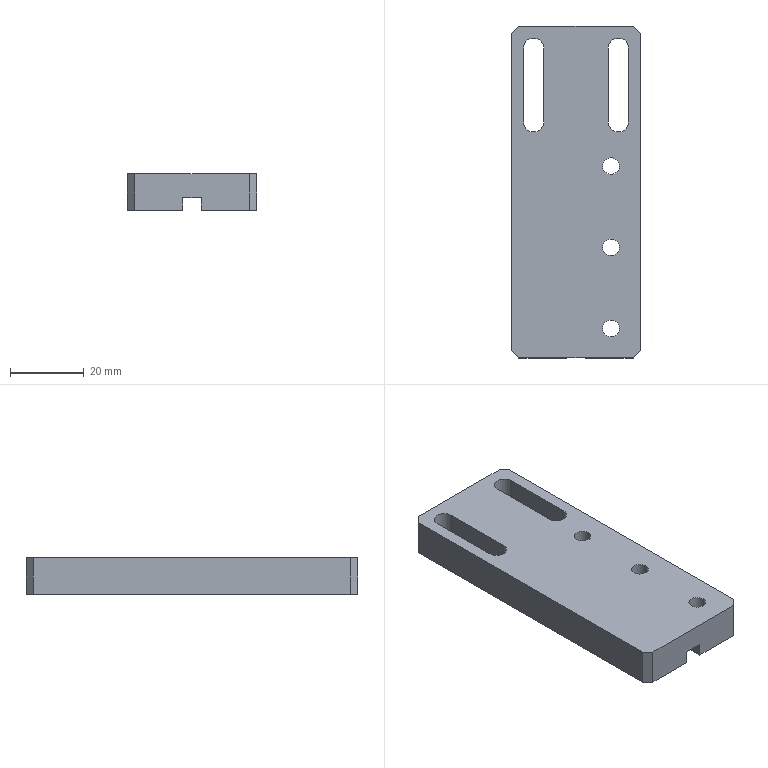Part | STEP file | 11-FG-B03611 | 1 solid | 37 faces | box 35 x 90 x 10 mm | volume 26239 mm3 | plane 21 | cylinder 16 | commonest cylinder face diameters 4.5 x6 8 x6 5.5 x4
STEP:
#1=CARTESIAN_POINT('',(13.5,-37.,4.4));
#2=VERTEX_POINT('',#1);
#3=CARTESIAN_POINT('',(5.5,-37.,4.4));
#4=VERTEX_POINT('',#3);
#5=CARTESIAN_POINT('',(9.5,-37.,4.4));
#6=DIRECTION('',(0.,0.,-1.));
#7=DIRECTION('',(-1.,0.,0.));
#8=AXIS2_PLACEMENT_3D('',#5,#6,#7);
#9=CIRCLE('',#8,4.);
#10=EDGE_CURVE('',#2,#4,#9,.T.);
#11=ORIENTED_EDGE('',*,*,#10,.F.);
#12=CARTESIAN_POINT('',(13.5,-37.,0.));
#13=VERTEX_POINT('',#12);
#14=CARTESIAN_POINT('',(13.5,-37.,0.));
#15=DIRECTION('',(0.,0.,-1.));
#16=VECTOR('',#15,1000.);
#17=LINE('',#14,#16);
#18=EDGE_CURVE('',#2,#13,#17,.T.);
#19=ORIENTED_EDGE('',*,*,#18,.T.);
#20=CARTESIAN_POINT('',(5.5,-37.,0.));
#21=VERTEX_POINT('',#20);
#22=CARTESIAN_POINT('',(9.5,-37.,0.));
#23=DIRECTION('',(0.,0.,-1.));
#24=DIRECTION('',(-1.,0.,0.));
#25=AXIS2_PLACEMENT_3D('',#22,#23,#24);
#26=CIRCLE('',#25,4.);
#27=EDGE_CURVE('',#13,#21,#26,.T.);
#28=ORIENTED_EDGE('',*,*,#27,.T.);
#29=CARTESIAN_POINT('',(5.5,-37.,0.));
#30=DIRECTION('',(0.,0.,-1.));
#31=VECTOR('',#30,1000.);
#32=LINE('',#29,#31);
#33=EDGE_CURVE('',#4,#21,#32,.T.);
#34=ORIENTED_EDGE('',*,*,#33,.F.);
#35=EDGE_LOOP('',(#11,#19,#28,#34));
#36=FACE_OUTER_BOUND('',#35,.T.);
#37=CARTESIAN_POINT('',(9.5,-37.,0.));
#38=DIRECTION('',(0.,0.,-1.));
#39=DIRECTION('',(-1.,0.,0.));
#40=AXIS2_PLACEMENT_3D('',#37,#38,#39);
#41=CYLINDRICAL_SURFACE('',#40,4.);
#42=ADVANCED_FACE('',(#36),#41,.F.);
#43=CARTESIAN_POINT('',(11.75,-37.,10.));
#44=VERTEX_POINT('',#43);
#45=CARTESIAN_POINT('',(7.25,-37.,10.));
#46=VERTEX_POINT('',#45);
#47=CARTESIAN_POINT('',(9.5,-37.,10.));
#48=DIRECTION('',(0.,0.,-1.));
#49=DIRECTION('',(-1.,0.,0.));
#50=AXIS2_PLACEMENT_3D('',#47,#48,#49);
#51=CIRCLE('',#50,2.25);
#52=EDGE_CURVE('',#44,#46,#51,.T.);
#53=ORIENTED_EDGE('',*,*,#52,.F.);
#54=CARTESIAN_POINT('',(11.75,-37.,4.4));
#55=VERTEX_POINT('',#54);
#56=CARTESIAN_POINT('',(11.75,-37.,0.));
#57=DIRECTION('',(0.,0.,-1.));
#58=VECTOR('',#57,1000.);
#59=LINE('',#56,#58);
#60=EDGE_CURVE('',#44,#55,#59,.T.);
#61=ORIENTED_EDGE('',*,*,#60,.T.);
#62=CARTESIAN_POINT('',(7.25,-37.,4.4));
#63=VERTEX_POINT('',#62);
#64=CARTESIAN_POINT('',(9.5,-37.,4.4));
#65=DIRECTION('',(0.,0.,-1.));
#66=DIRECTION('',(-1.,0.,0.));
#67=AXIS2_PLACEMENT_3D('',#64,#65,#66);
#68=CIRCLE('',#67,2.25);
#69=EDGE_CURVE('',#55,#63,#68,.T.);
#70=ORIENTED_EDGE('',*,*,#69,.T.);
#71=CARTESIAN_POINT('',(7.25,-37.,0.));
#72=DIRECTION('',(0.,0.,-1.));
#73=VECTOR('',#72,1000.);
#74=LINE('',#71,#73);
#75=EDGE_CURVE('',#46,#63,#74,.T.);
#76=ORIENTED_EDGE('',*,*,#75,.F.);
#77=EDGE_LOOP('',(#53,#61,#70,#76));
#78=FACE_OUTER_BOUND('',#77,.T.);
#79=CARTESIAN_POINT('',(9.5,-37.,0.));
#80=DIRECTION('',(0.,0.,-1.));
#81=DIRECTION('',(-1.,0.,0.));
#82=AXIS2_PLACEMENT_3D('',#79,#80,#81);
#83=CYLINDRICAL_SURFACE('',#82,2.25);
#84=ADVANCED_FACE('',(#78),#83,.F.);
#85=CARTESIAN_POINT('',(13.5,-15.,4.4));
#86=VERTEX_POINT('',#85);
#87=CARTESIAN_POINT('',(5.5,-15.,4.4));
#88=VERTEX_POINT('',#87);
#89=CARTESIAN_POINT('',(9.5,-15.,4.4));
#90=DIRECTION('',(0.,0.,-1.));
#91=DIRECTION('',(-1.,0.,0.));
#92=AXIS2_PLACEMENT_3D('',#89,#90,#91);
#93=CIRCLE('',#92,4.);
#94=EDGE_CURVE('',#86,#88,#93,.T.);
#95=ORIENTED_EDGE('',*,*,#94,.F.);
#96=CARTESIAN_POINT('',(13.5,-15.,0.));
#97=VERTEX_POINT('',#96);
#98=CARTESIAN_POINT('',(13.5,-15.,0.));
#99=DIRECTION('',(0.,0.,-1.));
#100=VECTOR('',#99,1000.);
#101=LINE('',#98,#100);
#102=EDGE_CURVE('',#86,#97,#101,.T.);
#103=ORIENTED_EDGE('',*,*,#102,.T.);
#104=CARTESIAN_POINT('',(5.5,-15.,0.));
#105=VERTEX_POINT('',#104);
#106=CARTESIAN_POINT('',(9.5,-15.,0.));
#107=DIRECTION('',(0.,0.,-1.));
#108=DIRECTION('',(-1.,0.,0.));
#109=AXIS2_PLACEMENT_3D('',#106,#107,#108);
#110=CIRCLE('',#109,4.);
#111=EDGE_CURVE('',#97,#105,#110,.T.);
#112=ORIENTED_EDGE('',*,*,#111,.T.);
#113=CARTESIAN_POINT('',(5.5,-15.,0.));
#114=DIRECTION('',(0.,0.,-1.));
#115=VECTOR('',#114,1000.);
#116=LINE('',#113,#115);
#117=EDGE_CURVE('',#88,#105,#116,.T.);
#118=ORIENTED_EDGE('',*,*,#117,.F.);
#119=EDGE_LOOP('',(#95,#103,#112,#118));
#120=FACE_OUTER_BOUND('',#119,.T.);
#121=CARTESIAN_POINT('',(9.5,-15.,0.));
#122=DIRECTION('',(0.,0.,-1.));
#123=DIRECTION('',(-1.,0.,0.));
#124=AXIS2_PLACEMENT_3D('',#121,#122,#123);
#125=CYLINDRICAL_SURFACE('',#124,4.);
#126=ADVANCED_FACE('',(#120),#125,.F.);
#127=CARTESIAN_POINT('',(11.75,-15.,10.));
#128=VERTEX_POINT('',#127);
#129=CARTESIAN_POINT('',(7.25,-15.,10.));
#130=VERTEX_POINT('',#129);
#131=CARTESIAN_POINT('',(9.5,-15.,10.));
#132=DIRECTION('',(0.,0.,-1.));
#133=DIRECTION('',(-1.,0.,0.));
#134=AXIS2_PLACEMENT_3D('',#131,#132,#133);
#135=CIRCLE('',#134,2.25);
#136=EDGE_CURVE('',#128,#130,#135,.T.);
#137=ORIENTED_EDGE('',*,*,#136,.F.);
#138=CARTESIAN_POINT('',(11.75,-15.,4.4));
#139=VERTEX_POINT('',#138);
#140=CARTESIAN_POINT('',(11.75,-15.,0.));
#141=DIRECTION('',(0.,0.,-1.));
#142=VECTOR('',#141,1000.);
#143=LINE('',#140,#142);
#144=EDGE_CURVE('',#128,#139,#143,.T.);
#145=ORIENTED_EDGE('',*,*,#144,.T.);
#146=CARTESIAN_POINT('',(7.25,-15.,4.4));
#147=VERTEX_POINT('',#146);
#148=CARTESIAN_POINT('',(9.5,-15.,4.4));
#149=DIRECTION('',(0.,0.,-1.));
#150=DIRECTION('',(-1.,0.,0.));
#151=AXIS2_PLACEMENT_3D('',#148,#149,#150);
#152=CIRCLE('',#151,2.25);
#153=EDGE_CURVE('',#139,#147,#152,.T.);
#154=ORIENTED_EDGE('',*,*,#153,.T.);
#155=CARTESIAN_POINT('',(7.25,-15.,0.));
#156=DIRECTION('',(0.,0.,-1.));
#157=VECTOR('',#156,1000.);
#158=LINE('',#155,#157);
#159=EDGE_CURVE('',#130,#147,#158,.T.);
#160=ORIENTED_EDGE('',*,*,#159,.F.);
#161=EDGE_LOOP('',(#137,#145,#154,#160));
#162=FACE_OUTER_BOUND('',#161,.T.);
#163=CARTESIAN_POINT('',(9.5,-15.,0.));
#164=DIRECTION('',(0.,0.,-1.));
#165=DIRECTION('',(-1.,0.,0.));
#166=AXIS2_PLACEMENT_3D('',#163,#164,#165);
#167=CYLINDRICAL_SURFACE('',#166,2.25);
#168=ADVANCED_FACE('',(#162),#167,.F.);
#169=CARTESIAN_POINT('',(13.5,7.,4.4));
#170=VERTEX_POINT('',#169);
#171=CARTESIAN_POINT('',(5.5,7.,4.4));
#172=VERTEX_POINT('',#171);
#173=CARTESIAN_POINT('',(9.5,7.,4.4));
#174=DIRECTION('',(0.,0.,-1.));
#175=DIRECTION('',(-1.,0.,0.));
#176=AXIS2_PLACEMENT_3D('',#173,#174,#175);
#177=CIRCLE('',#176,4.);
#178=EDGE_CURVE('',#170,#172,#177,.T.);
#179=ORIENTED_EDGE('',*,*,#178,.F.);
#180=CARTESIAN_POINT('',(13.5,7.,0.));
#181=VERTEX_POINT('',#180);
#182=CARTESIAN_POINT('',(13.5,7.,0.));
#183=DIRECTION('',(0.,0.,-1.));
#184=VECTOR('',#183,1000.);
#185=LINE('',#182,#184);
#186=EDGE_CURVE('',#170,#181,#185,.T.);
#187=ORIENTED_EDGE('',*,*,#186,.T.);
#188=CARTESIAN_POINT('',(5.5,7.,0.));
#189=VERTEX_POINT('',#188);
#190=CARTESIAN_POINT('',(9.5,7.,0.));
#191=DIRECTION('',(0.,0.,-1.));
#192=DIRECTION('',(-1.,0.,0.));
#193=AXIS2_PLACEMENT_3D('',#190,#191,#192);
#194=CIRCLE('',#193,4.);
#195=EDGE_CURVE('',#181,#189,#194,.T.);
#196=ORIENTED_EDGE('',*,*,#195,.T.);
#197=CARTESIAN_POINT('',(5.5,7.,0.));
#198=DIRECTION('',(0.,0.,-1.));
#199=VECTOR('',#198,1000.);
#200=LINE('',#197,#199);
#201=EDGE_CURVE('',#172,#189,#200,.T.);
#202=ORIENTED_EDGE('',*,*,#201,.F.);
#203=EDGE_LOOP('',(#179,#187,#196,#202));
#204=FACE_OUTER_BOUND('',#203,.T.);
#205=CARTESIAN_POINT('',(9.5,7.,0.));
#206=DIRECTION('',(0.,0.,-1.));
#207=DIRECTION('',(-1.,0.,0.));
#208=AXIS2_PLACEMENT_3D('',#205,#206,#207);
#209=CYLINDRICAL_SURFACE('',#208,4.);
#210=ADVANCED_FACE('',(#204),#209,.F.);
#211=CARTESIAN_POINT('',(11.75,7.,10.));
#212=VERTEX_POINT('',#211);
#213=CARTESIAN_POINT('',(7.25,7.,10.));
#214=VERTEX_POINT('',#213);
#215=CARTESIAN_POINT('',(9.5,7.,10.));
#216=DIRECTION('',(0.,0.,-1.));
#217=DIRECTION('',(-1.,0.,0.));
#218=AXIS2_PLACEMENT_3D('',#215,#216,#217);
#219=CIRCLE('',#218,2.25);
#220=EDGE_CURVE('',#212,#214,#219,.T.);
#221=ORIENTED_EDGE('',*,*,#220,.F.);
#222=CARTESIAN_POINT('',(11.75,7.,4.4));
#223=VERTEX_POINT('',#222);
#224=CARTESIAN_POINT('',(11.75,7.,0.));
#225=DIRECTION('',(0.,0.,-1.));
#226=VECTOR('',#225,1000.);
#227=LINE('',#224,#226);
#228=EDGE_CURVE('',#212,#223,#227,.T.);
#229=ORIENTED_EDGE('',*,*,#228,.T.);
#230=CARTESIAN_POINT('',(7.25,7.,4.4));
#231=VERTEX_POINT('',#230);
#232=CARTESIAN_POINT('',(9.5,7.,4.4));
#233=DIRECTION('',(0.,0.,-1.));
#234=DIRECTION('',(-1.,0.,0.));
#235=AXIS2_PLACEMENT_3D('',#232,#233,#234);
#236=CIRCLE('',#235,2.25);
#237=EDGE_CURVE('',#223,#231,#236,.T.);
#238=ORIENTED_EDGE('',*,*,#237,.T.);
#239=CARTESIAN_POINT('',(7.25,7.,0.));
#240=DIRECTION('',(0.,0.,-1.));
#241=VECTOR('',#240,1000.);
#242=LINE('',#239,#241);
#243=EDGE_CURVE('',#214,#231,#242,.T.);
#244=ORIENTED_EDGE('',*,*,#243,.F.);
#245=EDGE_LOOP('',(#221,#229,#238,#244));
#246=FACE_OUTER_BOUND('',#245,.T.);
#247=CARTESIAN_POINT('',(9.5,7.,0.));
#248=DIRECTION('',(0.,0.,-1.));
#249=DIRECTION('',(-1.,0.,0.));
#250=AXIS2_PLACEMENT_3D('',#247,#248,#249);
#251=CYLINDRICAL_SURFACE('',#250,2.25);
#252=ADVANCED_FACE('',(#246),#251,.F.);
#253=CARTESIAN_POINT('',(14.25,19.,0.));
#254=VERTEX_POINT('',#253);
#255=CARTESIAN_POINT('',(8.75,19.,0.));
#256=VERTEX_POINT('',#255);
#257=CARTESIAN_POINT('',(11.5,19.,0.));
#258=DIRECTION('',(0.,0.,-1.));
#259=DIRECTION('',(-1.,0.,0.));
#260=AXIS2_PLACEMENT_3D('',#257,#258,#259);
#261=CIRCLE('',#260,2.75);
#262=EDGE_CURVE('',#254,#256,#261,.T.);
#263=ORIENTED_EDGE('',*,*,#262,.F.);
#264=CARTESIAN_POINT('',(14.25,39.,0.));
#265=VERTEX_POINT('',#264);
#266=CARTESIAN_POINT('',(14.25,0.,0.));
#267=DIRECTION('',(0.,-1.,0.));
#268=VECTOR('',#267,1000.);
#269=LINE('',#266,#268);
#270=EDGE_CURVE('',#265,#254,#269,.T.);
#271=ORIENTED_EDGE('',*,*,#270,.F.);
#272=CARTESIAN_POINT('',(8.75,39.,0.));
#273=VERTEX_POINT('',#272);
#274=CARTESIAN_POINT('',(11.5,39.,0.));
#275=DIRECTION('',(0.,0.,-1.));
#276=DIRECTION('',(-1.,0.,0.));
#277=AXIS2_PLACEMENT_3D('',#274,#275,#276);
#278=CIRCLE('',#277,2.75);
#279=EDGE_CURVE('',#273,#265,#278,.T.);
#280=ORIENTED_EDGE('',*,*,#279,.F.);
#281=CARTESIAN_POINT('',(8.75,0.,0.));
#282=DIRECTION('',(0.,1.,0.));
#283=VECTOR('',#282,1000.);
#284=LINE('',#281,#283);
#285=EDGE_CURVE('',#256,#273,#284,.T.);
#286=ORIENTED_EDGE('',*,*,#285,.F.);
#287=EDGE_LOOP('',(#263,#271,#280,#286));
#288=FACE_BOUND('',#287,.T.);
#289=CARTESIAN_POINT('',(2.5,45.,0.));
#290=VERTEX_POINT('',#289);
#291=CARTESIAN_POINT('',(2.5,-45.,0.));
#292=VERTEX_POINT('',#291);
#293=CARTESIAN_POINT('',(2.5,0.,0.));
#294=DIRECTION('',(0.,-1.,0.));
#295=VECTOR('',#294,1000.);
#296=LINE('',#293,#295);
#297=EDGE_CURVE('',#290,#292,#296,.T.);
#298=ORIENTED_EDGE('',*,*,#297,.F.);
#299=CARTESIAN_POINT('',(15.5,45.,0.));
#300=VERTEX_POINT('',#299);
#301=CARTESIAN_POINT('',(17.5,45.,0.));
#302=DIRECTION('',(-1.,0.,0.));
#303=VECTOR('',#302,1000.);
#304=LINE('',#301,#303);
#305=EDGE_CURVE('',#300,#290,#304,.T.);
#306=ORIENTED_EDGE('',*,*,#305,.F.);
#307=CARTESIAN_POINT('',(17.5,43.,0.));
#308=VERTEX_POINT('',#307);
#309=CARTESIAN_POINT('',(30.25,30.25,0.));
#310=DIRECTION('',(0.7071,-0.7071,0.));
#311=VECTOR('',#310,1000.);
#312=LINE('',#309,#311);
#313=EDGE_CURVE('',#300,#308,#312,.T.);
#314=ORIENTED_EDGE('',*,*,#313,.T.);
#315=CARTESIAN_POINT('',(17.5,-43.,0.));
#316=VERTEX_POINT('',#315);
#317=CARTESIAN_POINT('',(17.5,45.,0.));
#318=DIRECTION('',(0.,1.,0.));
#319=VECTOR('',#318,1000.);
#320=LINE('',#317,#319);
#321=EDGE_CURVE('',#316,#308,#320,.T.);
#322=ORIENTED_EDGE('',*,*,#321,.F.);
#323=CARTESIAN_POINT('',(15.5,-45.,0.));
#324=VERTEX_POINT('',#323);
#325=CARTESIAN_POINT('',(30.25,-30.25,0.));
#326=DIRECTION('',(-0.7071,-0.7071,0.));
#327=VECTOR('',#326,1000.);
#328=LINE('',#325,#327);
#329=EDGE_CURVE('',#316,#324,#328,.T.);
#330=ORIENTED_EDGE('',*,*,#329,.T.);
#331=CARTESIAN_POINT('',(17.5,-45.,0.));
#332=DIRECTION('',(1.,0.,0.));
#333=VECTOR('',#332,1000.);
#334=LINE('',#331,#333);
#335=EDGE_CURVE('',#292,#324,#334,.T.);
#336=ORIENTED_EDGE('',*,*,#335,.F.);
#337=EDGE_LOOP('',(#298,#306,#314,#322,#330,#336));
#338=FACE_OUTER_BOUND('',#337,.T.);
#339=CARTESIAN_POINT('',(9.5,-37.,0.));
#340=DIRECTION('',(0.,0.,-1.));
#341=DIRECTION('',(-1.,0.,0.));
#342=AXIS2_PLACEMENT_3D('',#339,#340,#341);
#343=CIRCLE('',#342,4.);
#344=EDGE_CURVE('',#21,#13,#343,.T.);
#345=ORIENTED_EDGE('',*,*,#344,.F.);
#346=ORIENTED_EDGE('',*,*,#27,.F.);
#347=EDGE_LOOP('',(#345,#346));
#348=FACE_BOUND('',#347,.T.);
#349=CARTESIAN_POINT('',(9.5,-15.,0.));
#350=DIRECTION('',(0.,0.,-1.));
#351=DIRECTION('',(-1.,0.,0.));
#352=AXIS2_PLACEMENT_3D('',#349,#350,#351);
#353=CIRCLE('',#352,4.);
#354=EDGE_CURVE('',#105,#97,#353,.T.);
#355=ORIENTED_EDGE('',*,*,#354,.F.);
#356=ORIENTED_EDGE('',*,*,#111,.F.);
#357=EDGE_LOOP('',(#355,#356));
#358=FACE_BOUND('',#357,.T.);
#359=CARTESIAN_POINT('',(9.5,7.,0.));
#360=DIRECTION('',(0.,0.,-1.));
#361=DIRECTION('',(-1.,0.,0.));
#362=AXIS2_PLACEMENT_3D('',#359,#360,#361);
#363=CIRCLE('',#362,4.);
#364=EDGE_CURVE('',#189,#181,#363,.T.);
#365=ORIENTED_EDGE('',*,*,#364,.F.);
#366=ORIENTED_EDGE('',*,*,#195,.F.);
#367=EDGE_LOOP('',(#365,#366));
#368=FACE_BOUND('',#367,.T.);
#369=CARTESIAN_POINT('',(0.,0.,0.));
#370=DIRECTION('',(0.,0.,-1.));
#371=DIRECTION('',(-1.,0.,0.));
#372=AXIS2_PLACEMENT_3D('',#369,#370,#371);
#373=PLANE('',#372);
#374=ADVANCED_FACE('',(#288,#338,#348,#358,#368),#373,.T.);
#375=CARTESIAN_POINT('',(-17.5,43.,10.));
#376=VERTEX_POINT('',#375);
#377=CARTESIAN_POINT('',(-17.5,-43.,10.));
#378=VERTEX_POINT('',#377);
#379=CARTESIAN_POINT('',(-17.5,45.,10.));
#380=DIRECTION('',(0.,-1.,0.));
#381=VECTOR('',#380,1000.);
#382=LINE('',#379,#381);
#383=EDGE_CURVE('',#376,#378,#382,.T.);
#384=ORIENTED_EDGE('',*,*,#383,.F.);
#385=CARTESIAN_POINT('',(-17.5,43.,0.));
#386=VERTEX_POINT('',#385);
#387=CARTESIAN_POINT('',(-17.5,43.,10.));
#388=DIRECTION('',(0.,0.,-1.));
#389=VECTOR('',#388,1000.);
#390=LINE('',#387,#389);
#391=EDGE_CURVE('',#376,#386,#390,.T.);
#392=ORIENTED_EDGE('',*,*,#391,.T.);
#393=CARTESIAN_POINT('',(-17.5,-43.,0.));
#394=VERTEX_POINT('',#393);
#395=CARTESIAN_POINT('',(-17.5,45.,0.));
#396=DIRECTION('',(0.,-1.,0.));
#397=VECTOR('',#396,1000.);
#398=LINE('',#395,#397);
#399=EDGE_CURVE('',#386,#394,#398,.T.);
#400=ORIENTED_EDGE('',*,*,#399,.T.);
#401=CARTESIAN_POINT('',(-17.5,-43.,10.));
#402=DIRECTION('',(0.,0.,1.));
#403=VECTOR('',#402,1000.);
#404=LINE('',#401,#403);
#405=EDGE_CURVE('',#394,#378,#404,.T.);
#406=ORIENTED_EDGE('',*,*,#405,.T.);
#407=EDGE_LOOP('',(#384,#392,#400,#406));
#408=FACE_OUTER_BOUND('',#407,.T.);
#409=CARTESIAN_POINT('',(-17.5,45.,10.));
#410=DIRECTION('',(1.,0.,0.));
#411=DIRECTION('',(0.,1.,0.));
#412=AXIS2_PLACEMENT_3D('',#409,#410,#411);
#413=PLANE('',#412);
#414=ADVANCED_FACE('',(#408),#413,.F.);
#415=CARTESIAN_POINT('',(2.5,-45.,3.5));
#416=VERTEX_POINT('',#415);
#417=CARTESIAN_POINT('',(-2.5,-45.,3.5));
#418=VERTEX_POINT('',#417);
#419=CARTESIAN_POINT('',(-2.5,-45.,3.5));
#420=DIRECTION('',(-1.,0.,0.));
#421=VECTOR('',#420,1000.);
#422=LINE('',#419,#421);
#423=EDGE_CURVE('',#416,#418,#422,.T.);
#424=ORIENTED_EDGE('',*,*,#423,.F.);
#425=CARTESIAN_POINT('',(2.5,-45.,3.5));
#426=DIRECTION('',(0.,0.,1.));
#427=VECTOR('',#426,1000.);
#428=LINE('',#425,#427);
#429=EDGE_CURVE('',#292,#416,#428,.T.);
#430=ORIENTED_EDGE('',*,*,#429,.F.);
#431=ORIENTED_EDGE('',*,*,#335,.T.);
#432=CARTESIAN_POINT('',(15.5,-45.,10.));
#433=VERTEX_POINT('',#432);
#434=CARTESIAN_POINT('',(15.5,-45.,10.));
#435=DIRECTION('',(0.,0.,1.));
#436=VECTOR('',#435,1000.);
#437=LINE('',#434,#436);
#438=EDGE_CURVE('',#324,#433,#437,.T.);
#439=ORIENTED_EDGE('',*,*,#438,.T.);
#440=CARTESIAN_POINT('',(-15.5,-45.,10.));
#441=VERTEX_POINT('',#440);
#442=CARTESIAN_POINT('',(17.5,-45.,10.));
#443=DIRECTION('',(1.,0.,0.));
#444=VECTOR('',#443,1000.);
#445=LINE('',#442,#444);
#446=EDGE_CURVE('',#441,#433,#445,.T.);
#447=ORIENTED_EDGE('',*,*,#446,.F.);
#448=CARTESIAN_POINT('',(-15.5,-45.,0.));
#449=VERTEX_POINT('',#448);
#450=CARTESIAN_POINT('',(-15.5,-45.,10.));
#451=DIRECTION('',(0.,0.,-1.));
#452=VECTOR('',#451,1000.);
#453=LINE('',#450,#452);
#454=EDGE_CURVE('',#441,#449,#453,.T.);
#455=ORIENTED_EDGE('',*,*,#454,.T.);
#456=CARTESIAN_POINT('',(-2.5,-45.,0.));
#457=VERTEX_POINT('',#456);
#458=CARTESIAN_POINT('',(17.5,-45.,0.));
#459=DIRECTION('',(1.,0.,0.));
#460=VECTOR('',#459,1000.);
#461=LINE('',#458,#460);
#462=EDGE_CURVE('',#449,#457,#461,.T.);
#463=ORIENTED_EDGE('',*,*,#462,.T.);
#464=CARTESIAN_POINT('',(-2.5,-45.,3.5));
#465=DIRECTION('',(0.,0.,-1.));
#466=VECTOR('',#465,1000.);
#467=LINE('',#464,#466);
#468=EDGE_CURVE('',#418,#457,#467,.T.);
#469=ORIENTED_EDGE('',*,*,#468,.F.);
#470=EDGE_LOOP('',(#424,#430,#431,#439,#447,#455,#463,#469));
#471=FACE_OUTER_BOUND('',#470,.T.);
#472=CARTESIAN_POINT('',(17.5,-45.,10.));
#473=DIRECTION('',(0.,1.,0.));
#474=DIRECTION('',(-1.,0.,0.));
#475=AXIS2_PLACEMENT_3D('',#472,#473,#474);
#476=PLANE('',#475);
#477=ADVANCED_FACE('',(#471),#476,.F.);
#478=ORIENTED_EDGE('',*,*,#321,.T.);
#479=CARTESIAN_POINT('',(17.5,43.,10.));
#480=VERTEX_POINT('',#479);
#481=CARTESIAN_POINT('',(17.5,43.,10.));
#482=DIRECTION('',(0.,0.,1.));
#483=VECTOR('',#482,1000.);
#484=LINE('',#481,#483);
#485=EDGE_CURVE('',#308,#480,#484,.T.);
#486=ORIENTED_EDGE('',*,*,#485,.T.);
#487=CARTESIAN_POINT('',(17.5,-43.,10.));
#488=VERTEX_POINT('',#487);
#489=CARTESIAN_POINT('',(17.5,45.,10.));
#490=DIRECTION('',(0.,1.,0.));
#491=VECTOR('',#490,1000.);
#492=LINE('',#489,#491);
#493=EDGE_CURVE('',#488,#480,#492,.T.);
#494=ORIENTED_EDGE('',*,*,#493,.F.);
#495=CARTESIAN_POINT('',(17.5,-43.,10.));
#496=DIRECTION('',(0.,0.,-1.));
#497=VECTOR('',#496,1000.);
#498=LINE('',#495,#497);
#499=EDGE_CURVE('',#488,#316,#498,.T.);
#500=ORIENTED_EDGE('',*,*,#499,.T.);
#501=EDGE_LOOP('',(#478,#486,#494,#500));
#502=FACE_OUTER_BOUND('',#501,.T.);
#503=CARTESIAN_POINT('',(17.5,45.,10.));
#504=DIRECTION('',(-1.,0.,0.));
#505=DIRECTION('',(0.,-1.,0.));
#506=AXIS2_PLACEMENT_3D('',#503,#504,#505);
#507=PLANE('',#506);
#508=ADVANCED_FACE('',(#502),#507,.F.);
#509=ORIENTED_EDGE('',*,*,#305,.T.);
#510=CARTESIAN_POINT('',(2.5,45.,3.5));
#511=VERTEX_POINT('',#510);
#512=CARTESIAN_POINT('',(2.5,45.,10.));
#513=DIRECTION('',(0.,0.,1.));
#514=VECTOR('',#513,1000.);
#515=LINE('',#512,#514);
#516=EDGE_CURVE('',#290,#511,#515,.T.);
#517=ORIENTED_EDGE('',*,*,#516,.T.);
#518=CARTESIAN_POINT('',(-2.5,45.,3.5));
#519=VERTEX_POINT('',#518);
#520=CARTESIAN_POINT('',(17.5,45.,3.5));
#521=DIRECTION('',(-1.,0.,0.));
#522=VECTOR('',#521,1000.);
#523=LINE('',#520,#522);
#524=EDGE_CURVE('',#511,#519,#523,.T.);
#525=ORIENTED_EDGE('',*,*,#524,.T.);
#526=CARTESIAN_POINT('',(-2.5,45.,0.));
#527=VERTEX_POINT('',#526);
#528=CARTESIAN_POINT('',(-2.5,45.,10.));
#529=DIRECTION('',(0.,0.,-1.));
#530=VECTOR('',#529,1000.);
#531=LINE('',#528,#530);
#532=EDGE_CURVE('',#519,#527,#531,.T.);
#533=ORIENTED_EDGE('',*,*,#532,.T.);
#534=CARTESIAN_POINT('',(-15.5,45.,0.));
#535=VERTEX_POINT('',#534);
#536=CARTESIAN_POINT('',(17.5,45.,0.));
#537=DIRECTION('',(-1.,0.,0.));
#538=VECTOR('',#537,1000.);
#539=LINE('',#536,#538);
#540=EDGE_CURVE('',#527,#535,#539,.T.);
#541=ORIENTED_EDGE('',*,*,#540,.T.);
#542=CARTESIAN_POINT('',(-15.5,45.,10.));
#543=VERTEX_POINT('',#542);
#544=CARTESIAN_POINT('',(-15.5,45.,10.));
#545=DIRECTION('',(0.,0.,1.));
#546=VECTOR('',#545,1000.);
#547=LINE('',#544,#546);
#548=EDGE_CURVE('',#535,#543,#547,.T.);
#549=ORIENTED_EDGE('',*,*,#548,.T.);
#550=CARTESIAN_POINT('',(15.5,45.,10.));
#551=VERTEX_POINT('',#550);
#552=CARTESIAN_POINT('',(17.5,45.,10.));
#553=DIRECTION('',(-1.,0.,0.));
#554=VECTOR('',#553,1000.);
#555=LINE('',#552,#554);
#556=EDGE_CURVE('',#551,#543,#555,.T.);
#557=ORIENTED_EDGE('',*,*,#556,.F.);
#558=CARTESIAN_POINT('',(15.5,45.,10.));
#559=DIRECTION('',(0.,0.,-1.));
#560=VECTOR('',#559,1000.);
#561=LINE('',#558,#560);
#562=EDGE_CURVE('',#551,#300,#561,.T.);
#563=ORIENTED_EDGE('',*,*,#562,.T.);
#564=EDGE_LOOP('',(#509,#517,#525,#533,#541,#549,#557,#563));
#565=FACE_OUTER_BOUND('',#564,.T.);
#566=CARTESIAN_POINT('',(17.5,45.,10.));
#567=DIRECTION('',(0.,-1.,0.));
#568=DIRECTION('',(1.,0.,0.));
#569=AXIS2_PLACEMENT_3D('',#566,#567,#568);
#570=PLANE('',#569);
#571=ADVANCED_FACE('',(#565),#570,.F.);
#572=CARTESIAN_POINT('',(-8.75,19.,10.));
#573=VERTEX_POINT('',#572);
#574=CARTESIAN_POINT('',(-8.75,39.,10.));
#575=VERTEX_POINT('',#574);
#576=CARTESIAN_POINT('',(-8.75,19.,10.));
#577=DIRECTION('',(0.,1.,0.));
#578=VECTOR('',#577,1000.);
#579=LINE('',#576,#578);
#580=EDGE_CURVE('',#573,#575,#579,.T.);
#581=ORIENTED_EDGE('',*,*,#580,.F.);
#582=CARTESIAN_POINT('',(-14.25,19.,10.));
#583=VERTEX_POINT('',#582);
#584=CARTESIAN_POINT('',(-11.5,19.,10.));
#585=DIRECTION('',(0.,0.,1.));
#586=DIRECTION('',(1.,0.,0.));
#587=AXIS2_PLACEMENT_3D('',#584,#585,#586);
#588=CIRCLE('',#587,2.75);
#589=EDGE_CURVE('',#583,#573,#588,.T.);
#590=ORIENTED_EDGE('',*,*,#589,.F.);
#591=CARTESIAN_POINT('',(-14.25,39.,10.));
#592=VERTEX_POINT('',#591);
#593=CARTESIAN_POINT('',(-14.25,19.,10.));
#594=DIRECTION('',(0.,-1.,0.));
#595=VECTOR('',#594,1000.);
#596=LINE('',#593,#595);
#597=EDGE_CURVE('',#592,#583,#596,.T.);
#598=ORIENTED_EDGE('',*,*,#597,.F.);
#599=CARTESIAN_POINT('',(-11.5,39.,10.));
#600=DIRECTION('',(0.,0.,1.));
#601=DIRECTION('',(1.,0.,0.));
#602=AXIS2_PLACEMENT_3D('',#599,#600,#601);
#603=CIRCLE('',#602,2.75);
#604=EDGE_CURVE('',#575,#592,#603,.T.);
#605=ORIENTED_EDGE('',*,*,#604,.F.);
#606=EDGE_LOOP('',(#581,#590,#598,#605));
#607=FACE_BOUND('',#606,.T.);
#608=CARTESIAN_POINT('',(14.25,19.,10.));
#609=VERTEX_POINT('',#608);
#610=CARTESIAN_POINT('',(14.25,39.,10.));
#611=VERTEX_POINT('',#610);
#612=CARTESIAN_POINT('',(14.25,19.,10.));
#613=DIRECTION('',(0.,1.,0.));
#614=VECTOR('',#613,1000.);
#615=LINE('',#612,#614);
#616=EDGE_CURVE('',#609,#611,#615,.T.);
#617=ORIENTED_EDGE('',*,*,#616,.F.);
#618=CARTESIAN_POINT('',(8.75,19.,10.));
#619=VERTEX_POINT('',#618);
#620=CARTESIAN_POINT('',(11.5,19.,10.));
#621=DIRECTION('',(0.,0.,1.));
#622=DIRECTION('',(1.,0.,0.));
#623=AXIS2_PLACEMENT_3D('',#620,#621,#622);
#624=CIRCLE('',#623,2.75);
#625=EDGE_CURVE('',#619,#609,#624,.T.);
#626=ORIENTED_EDGE('',*,*,#625,.F.);
#627=CARTESIAN_POINT('',(8.75,39.,10.));
#628=VERTEX_POINT('',#627);
#629=CARTESIAN_POINT('',(8.75,19.,10.));
#630=DIRECTION('',(0.,-1.,0.));
#631=VECTOR('',#630,1000.);
#632=LINE('',#629,#631);
#633=EDGE_CURVE('',#628,#619,#632,.T.);
#634=ORIENTED_EDGE('',*,*,#633,.F.);
#635=CARTESIAN_POINT('',(11.5,39.,10.));
#636=DIRECTION('',(0.,0.,1.));
#637=DIRECTION('',(1.,0.,0.));
#638=AXIS2_PLACEMENT_3D('',#635,#636,#637);
#639=CIRCLE('',#638,2.75);
#640=EDGE_CURVE('',#611,#628,#639,.T.);
#641=ORIENTED_EDGE('',*,*,#640,.F.);
#642=EDGE_LOOP('',(#617,#626,#634,#641));
#643=FACE_BOUND('',#642,.T.);
#644=CARTESIAN_POINT('',(9.5,-37.,10.));
#645=DIRECTION('',(0.,0.,-1.));
#646=DIRECTION('',(-1.,0.,0.));
#647=AXIS2_PLACEMENT_3D('',#644,#645,#646);
#648=CIRCLE('',#647,2.25);
#649=EDGE_CURVE('',#46,#44,#648,.T.);
#650=ORIENTED_EDGE('',*,*,#649,.T.);
#651=ORIENTED_EDGE('',*,*,#52,.T.);
#652=EDGE_LOOP('',(#650,#651));
#653=FACE_BOUND('',#652,.T.);
#654=CARTESIAN_POINT('',(9.5,-15.,10.));
#655=DIRECTION('',(0.,0.,-1.));
#656=DIRECTION('',(-1.,0.,0.));
#657=AXIS2_PLACEMENT_3D('',#654,#655,#656);
#658=CIRCLE('',#657,2.25);
#659=EDGE_CURVE('',#130,#128,#658,.T.);
#660=ORIENTED_EDGE('',*,*,#659,.T.);
#661=ORIENTED_EDGE('',*,*,#136,.T.);
#662=EDGE_LOOP('',(#660,#661));
#663=FACE_BOUND('',#662,.T.);
#664=CARTESIAN_POINT('',(9.5,7.,10.));
#665=DIRECTION('',(0.,0.,-1.));
#666=DIRECTION('',(-1.,0.,0.));
#667=AXIS2_PLACEMENT_3D('',#664,#665,#666);
#668=CIRCLE('',#667,2.25);
#669=EDGE_CURVE('',#214,#212,#668,.T.);
#670=ORIENTED_EDGE('',*,*,#669,.T.);
#671=ORIENTED_EDGE('',*,*,#220,.T.);
#672=EDGE_LOOP('',(#670,#671));
#673=FACE_BOUND('',#672,.T.);
#674=ORIENTED_EDGE('',*,*,#493,.T.);
#675=CARTESIAN_POINT('',(15.5,45.,10.));
#676=DIRECTION('',(-0.7071,0.7071,0.));
#677=VECTOR('',#676,1000.);
#678=LINE('',#675,#677);
#679=EDGE_CURVE('',#480,#551,#678,.T.);
#680=ORIENTED_EDGE('',*,*,#679,.T.);
#681=ORIENTED_EDGE('',*,*,#556,.T.);
#682=CARTESIAN_POINT('',(-17.5,43.,10.));
#683=DIRECTION('',(-0.7071,-0.7071,0.));
#684=VECTOR('',#683,1000.);
#685=LINE('',#682,#684);
#686=EDGE_CURVE('',#543,#376,#685,.T.);
#687=ORIENTED_EDGE('',*,*,#686,.T.);
#688=ORIENTED_EDGE('',*,*,#383,.T.);
#689=CARTESIAN_POINT('',(-15.5,-45.,10.));
#690=DIRECTION('',(0.7071,-0.7071,0.));
#691=VECTOR('',#690,1000.);
#692=LINE('',#689,#691);
#693=EDGE_CURVE('',#378,#441,#692,.T.);
#694=ORIENTED_EDGE('',*,*,#693,.T.);
#695=ORIENTED_EDGE('',*,*,#446,.T.);
#696=CARTESIAN_POINT('',(17.5,-43.,10.));
#697=DIRECTION('',(0.7071,0.7071,0.));
#698=VECTOR('',#697,1000.);
#699=LINE('',#696,#698);
#700=EDGE_CURVE('',#433,#488,#699,.T.);
#701=ORIENTED_EDGE('',*,*,#700,.T.);
#702=EDGE_LOOP('',(#674,#680,#681,#687,#688,#694,#695,#701));
#703=FACE_OUTER_BOUND('',#702,.T.);
#704=CARTESIAN_POINT('',(0.,0.,10.));
#705=DIRECTION('',(0.,0.,-1.));
#706=DIRECTION('',(-1.,0.,0.));
#707=AXIS2_PLACEMENT_3D('',#704,#705,#706);
#708=PLANE('',#707);
#709=ADVANCED_FACE('',(#607,#643,#653,#663,#673,#703),#708,.F.);
#710=CARTESIAN_POINT('',(-8.75,19.,0.));
#711=VERTEX_POINT('',#710);
#712=CARTESIAN_POINT('',(-14.25,19.,0.));
#713=VERTEX_POINT('',#712);
#714=CARTESIAN_POINT('',(-11.5,19.,0.));
#715=DIRECTION('',(0.,0.,-1.));
#716=DIRECTION('',(-1.,0.,0.));
#717=AXIS2_PLACEMENT_3D('',#714,#715,#716);
#718=CIRCLE('',#717,2.75);
#719=EDGE_CURVE('',#711,#713,#718,.T.);
#720=ORIENTED_EDGE('',*,*,#719,.F.);
#721=CARTESIAN_POINT('',(-8.75,39.,0.));
#722=VERTEX_POINT('',#721);
#723=CARTESIAN_POINT('',(-8.75,0.,0.));
#724=DIRECTION('',(0.,-1.,0.));
#725=VECTOR('',#724,1000.);
#726=LINE('',#723,#725);
#727=EDGE_CURVE('',#722,#711,#726,.T.);
#728=ORIENTED_EDGE('',*,*,#727,.F.);
#729=CARTESIAN_POINT('',(-14.25,39.,0.));
#730=VERTEX_POINT('',#729);
#731=CARTESIAN_POINT('',(-11.5,39.,0.));
#732=DIRECTION('',(0.,0.,-1.));
#733=DIRECTION('',(-1.,0.,0.));
#734=AXIS2_PLACEMENT_3D('',#731,#732,#733);
#735=CIRCLE('',#734,2.75);
#736=EDGE_CURVE('',#730,#722,#735,.T.);
#737=ORIENTED_EDGE('',*,*,#736,.F.);
#738=CARTESIAN_POINT('',(-14.25,0.,0.));
#739=DIRECTION('',(0.,1.,0.));
#740=VECTOR('',#739,1000.);
#741=LINE('',#738,#740);
#742=EDGE_CURVE('',#713,#730,#741,.T.);
#743=ORIENTED_EDGE('',*,*,#742,.F.);
#744=EDGE_LOOP('',(#720,#728,#737,#743));
#745=FACE_BOUND('',#744,.T.);
#746=CARTESIAN_POINT('',(-2.5,0.,0.));
#747=DIRECTION('',(0.,1.,0.));
#748=VECTOR('',#747,1000.);
#749=LINE('',#746,#748);
#750=EDGE_CURVE('',#457,#527,#749,.T.);
#751=ORIENTED_EDGE('',*,*,#750,.F.);
#752=ORIENTED_EDGE('',*,*,#462,.F.);
#753=CARTESIAN_POINT('',(-30.25,-30.25,0.));
#754=DIRECTION('',(-0.7071,0.7071,0.));
#755=VECTOR('',#754,1000.);
#756=LINE('',#753,#755);
#757=EDGE_CURVE('',#449,#394,#756,.T.);
#758=ORIENTED_EDGE('',*,*,#757,.T.);
#759=ORIENTED_EDGE('',*,*,#399,.F.);
#760=CARTESIAN_POINT('',(-30.25,30.25,0.));
#761=DIRECTION('',(0.7071,0.7071,0.));
#762=VECTOR('',#761,1000.);
#763=LINE('',#760,#762);
#764=EDGE_CURVE('',#386,#535,#763,.T.);
#765=ORIENTED_EDGE('',*,*,#764,.T.);
#766=ORIENTED_EDGE('',*,*,#540,.F.);
#767=EDGE_LOOP('',(#751,#752,#758,#759,#765,#766));
#768=FACE_OUTER_BOUND('',#767,.T.);
#769=CARTESIAN_POINT('',(0.,0.,0.));
#770=DIRECTION('',(0.,0.,-1.));
#771=DIRECTION('',(-1.,0.,0.));
#772=AXIS2_PLACEMENT_3D('',#769,#770,#771);
#773=PLANE('',#772);
#774=ADVANCED_FACE('',(#745,#768),#773,.T.);
#775=ORIENTED_EDGE('',*,*,#228,.F.);
#776=ORIENTED_EDGE('',*,*,#669,.F.);
#777=ORIENTED_EDGE('',*,*,#243,.T.);
#778=CARTESIAN_POINT('',(9.5,7.,4.4));
#779=DIRECTION('',(0.,0.,-1.));
#780=DIRECTION('',(-1.,0.,0.));
#781=AXIS2_PLACEMENT_3D('',#778,#779,#780);
#782=CIRCLE('',#781,2.25);
#783=EDGE_CURVE('',#231,#223,#782,.T.);
#784=ORIENTED_EDGE('',*,*,#783,.T.);
#785=EDGE_LOOP('',(#775,#776,#777,#784));
#786=FACE_OUTER_BOUND('',#785,.T.);
#787=CARTESIAN_POINT('',(9.5,7.,0.));
#788=DIRECTION('',(0.,0.,-1.));
#789=DIRECTION('',(-1.,0.,0.));
#790=AXIS2_PLACEMENT_3D('',#787,#788,#789);
#791=CYLINDRICAL_SURFACE('',#790,2.25);
#792=ADVANCED_FACE('',(#786),#791,.F.);
#793=ORIENTED_EDGE('',*,*,#783,.F.);
#794=ORIENTED_EDGE('',*,*,#237,.F.);
#795=EDGE_LOOP('',(#793,#794));
#796=FACE_BOUND('',#795,.T.);
#797=CARTESIAN_POINT('',(9.5,7.,4.4));
#798=DIRECTION('',(0.,0.,-1.));
#799=DIRECTION('',(-1.,0.,0.));
#800=AXIS2_PLACEMENT_3D('',#797,#798,#799);
#801=CIRCLE('',#800,4.);
#802=EDGE_CURVE('',#172,#170,#801,.T.);
#803=ORIENTED_EDGE('',*,*,#802,.T.);
#804=ORIENTED_EDGE('',*,*,#178,.T.);
#805=EDGE_LOOP('',(#803,#804));
#806=FACE_OUTER_BOUND('',#805,.T.);
#807=CARTESIAN_POINT('',(11.75,7.,4.4));
#808=DIRECTION('',(0.,0.,1.));
#809=DIRECTION('',(1.,0.,0.));
#810=AXIS2_PLACEMENT_3D('',#807,#808,#809);
#811=PLANE('',#810);
#812=ADVANCED_FACE('',(#796,#806),#811,.F.);
#813=ORIENTED_EDGE('',*,*,#186,.F.);
#814=ORIENTED_EDGE('',*,*,#802,.F.);
#815=ORIENTED_EDGE('',*,*,#201,.T.);
#816=ORIENTED_EDGE('',*,*,#364,.T.);
#817=EDGE_LOOP('',(#813,#814,#815,#816));
#818=FACE_OUTER_BOUND('',#817,.T.);
#819=CARTESIAN_POINT('',(9.5,7.,0.));
#820=DIRECTION('',(0.,0.,-1.));
#821=DIRECTION('',(-1.,0.,0.));
#822=AXIS2_PLACEMENT_3D('',#819,#820,#821);
#823=CYLINDRICAL_SURFACE('',#822,4.);
#824=ADVANCED_FACE('',(#818),#823,.F.);
#825=ORIENTED_EDGE('',*,*,#144,.F.);
#826=ORIENTED_EDGE('',*,*,#659,.F.);
#827=ORIENTED_EDGE('',*,*,#159,.T.);
#828=CARTESIAN_POINT('',(9.5,-15.,4.4));
#829=DIRECTION('',(0.,0.,-1.));
#830=DIRECTION('',(-1.,0.,0.));
#831=AXIS2_PLACEMENT_3D('',#828,#829,#830);
#832=CIRCLE('',#831,2.25);
#833=EDGE_CURVE('',#147,#139,#832,.T.);
#834=ORIENTED_EDGE('',*,*,#833,.T.);
#835=EDGE_LOOP('',(#825,#826,#827,#834));
#836=FACE_OUTER_BOUND('',#835,.T.);
#837=CARTESIAN_POINT('',(9.5,-15.,0.));
#838=DIRECTION('',(0.,0.,-1.));
#839=DIRECTION('',(-1.,0.,0.));
#840=AXIS2_PLACEMENT_3D('',#837,#838,#839);
#841=CYLINDRICAL_SURFACE('',#840,2.25);
#842=ADVANCED_FACE('',(#836),#841,.F.);
#843=ORIENTED_EDGE('',*,*,#833,.F.);
#844=ORIENTED_EDGE('',*,*,#153,.F.);
#845=EDGE_LOOP('',(#843,#844));
#846=FACE_BOUND('',#845,.T.);
#847=CARTESIAN_POINT('',(9.5,-15.,4.4));
#848=DIRECTION('',(0.,0.,-1.));
#849=DIRECTION('',(-1.,0.,0.));
#850=AXIS2_PLACEMENT_3D('',#847,#848,#849);
#851=CIRCLE('',#850,4.);
#852=EDGE_CURVE('',#88,#86,#851,.T.);
#853=ORIENTED_EDGE('',*,*,#852,.T.);
#854=ORIENTED_EDGE('',*,*,#94,.T.);
#855=EDGE_LOOP('',(#853,#854));
#856=FACE_OUTER_BOUND('',#855,.T.);
#857=CARTESIAN_POINT('',(11.75,-15.,4.4));
#858=DIRECTION('',(0.,0.,1.));
#859=DIRECTION('',(1.,0.,0.));
#860=AXIS2_PLACEMENT_3D('',#857,#858,#859);
#861=PLANE('',#860);
#862=ADVANCED_FACE('',(#846,#856),#861,.F.);
#863=ORIENTED_EDGE('',*,*,#102,.F.);
#864=ORIENTED_EDGE('',*,*,#852,.F.);
#865=ORIENTED_EDGE('',*,*,#117,.T.);
#866=ORIENTED_EDGE('',*,*,#354,.T.);
#867=EDGE_LOOP('',(#863,#864,#865,#866));
#868=FACE_OUTER_BOUND('',#867,.T.);
#869=CARTESIAN_POINT('',(9.5,-15.,0.));
#870=DIRECTION('',(0.,0.,-1.));
#871=DIRECTION('',(-1.,0.,0.));
#872=AXIS2_PLACEMENT_3D('',#869,#870,#871);
#873=CYLINDRICAL_SURFACE('',#872,4.);
#874=ADVANCED_FACE('',(#868),#873,.F.);
#875=ORIENTED_EDGE('',*,*,#60,.F.);
#876=ORIENTED_EDGE('',*,*,#649,.F.);
#877=ORIENTED_EDGE('',*,*,#75,.T.);
#878=CARTESIAN_POINT('',(9.5,-37.,4.4));
#879=DIRECTION('',(0.,0.,-1.));
#880=DIRECTION('',(-1.,0.,0.));
#881=AXIS2_PLACEMENT_3D('',#878,#879,#880);
#882=CIRCLE('',#881,2.25);
#883=EDGE_CURVE('',#63,#55,#882,.T.);
#884=ORIENTED_EDGE('',*,*,#883,.T.);
#885=EDGE_LOOP('',(#875,#876,#877,#884));
#886=FACE_OUTER_BOUND('',#885,.T.);
#887=CARTESIAN_POINT('',(9.5,-37.,0.));
#888=DIRECTION('',(0.,0.,-1.));
#889=DIRECTION('',(-1.,0.,0.));
#890=AXIS2_PLACEMENT_3D('',#887,#888,#889);
#891=CYLINDRICAL_SURFACE('',#890,2.25);
#892=ADVANCED_FACE('',(#886),#891,.F.);
#893=ORIENTED_EDGE('',*,*,#883,.F.);
#894=ORIENTED_EDGE('',*,*,#69,.F.);
#895=EDGE_LOOP('',(#893,#894));
#896=FACE_BOUND('',#895,.T.);
#897=CARTESIAN_POINT('',(9.5,-37.,4.4));
#898=DIRECTION('',(0.,0.,-1.));
#899=DIRECTION('',(-1.,0.,0.));
#900=AXIS2_PLACEMENT_3D('',#897,#898,#899);
#901=CIRCLE('',#900,4.);
#902=EDGE_CURVE('',#4,#2,#901,.T.);
#903=ORIENTED_EDGE('',*,*,#902,.T.);
#904=ORIENTED_EDGE('',*,*,#10,.T.);
#905=EDGE_LOOP('',(#903,#904));
#906=FACE_OUTER_BOUND('',#905,.T.);
#907=CARTESIAN_POINT('',(11.75,-37.,4.4));
#908=DIRECTION('',(0.,0.,1.));
#909=DIRECTION('',(1.,0.,0.));
#910=AXIS2_PLACEMENT_3D('',#907,#908,#909);
#911=PLANE('',#910);
#912=ADVANCED_FACE('',(#896,#906),#911,.F.);
#913=ORIENTED_EDGE('',*,*,#18,.F.);
#914=ORIENTED_EDGE('',*,*,#902,.F.);
#915=ORIENTED_EDGE('',*,*,#33,.T.);
#916=ORIENTED_EDGE('',*,*,#344,.T.);
#917=EDGE_LOOP('',(#913,#914,#915,#916));
#918=FACE_OUTER_BOUND('',#917,.T.);
#919=CARTESIAN_POINT('',(9.5,-37.,0.));
#920=DIRECTION('',(0.,0.,-1.));
#921=DIRECTION('',(-1.,0.,0.));
#922=AXIS2_PLACEMENT_3D('',#919,#920,#921);
#923=CYLINDRICAL_SURFACE('',#922,4.);
#924=ADVANCED_FACE('',(#918),#923,.F.);
#925=ORIENTED_EDGE('',*,*,#679,.F.);
#926=ORIENTED_EDGE('',*,*,#485,.F.);
#927=ORIENTED_EDGE('',*,*,#313,.F.);
#928=ORIENTED_EDGE('',*,*,#562,.F.);
#929=EDGE_LOOP('',(#925,#926,#927,#928));
#930=FACE_OUTER_BOUND('',#929,.T.);
#931=CARTESIAN_POINT('',(15.5,45.,10.));
#932=DIRECTION('',(-0.7071,-0.7071,0.));
#933=DIRECTION('',(0.,0.,-1.));
#934=AXIS2_PLACEMENT_3D('',#931,#932,#933);
#935=PLANE('',#934);
#936=ADVANCED_FACE('',(#930),#935,.F.);
#937=ORIENTED_EDGE('',*,*,#686,.F.);
#938=ORIENTED_EDGE('',*,*,#548,.F.);
#939=ORIENTED_EDGE('',*,*,#764,.F.);
#940=ORIENTED_EDGE('',*,*,#391,.F.);
#941=EDGE_LOOP('',(#937,#938,#939,#940));
#942=FACE_OUTER_BOUND('',#941,.T.);
#943=CARTESIAN_POINT('',(-17.5,43.,10.));
#944=DIRECTION('',(0.7071,-0.7071,0.));
#945=DIRECTION('',(0.,0.,-1.));
#946=AXIS2_PLACEMENT_3D('',#943,#944,#945);
#947=PLANE('',#946);
#948=ADVANCED_FACE('',(#942),#947,.F.);
#949=ORIENTED_EDGE('',*,*,#693,.F.);
#950=ORIENTED_EDGE('',*,*,#405,.F.);
#951=ORIENTED_EDGE('',*,*,#757,.F.);
#952=ORIENTED_EDGE('',*,*,#454,.F.);
#953=EDGE_LOOP('',(#949,#950,#951,#952));
#954=FACE_OUTER_BOUND('',#953,.T.);
#955=CARTESIAN_POINT('',(-15.5,-45.,10.));
#956=DIRECTION('',(0.7071,0.7071,0.));
#957=DIRECTION('',(0.,0.,-1.));
#958=AXIS2_PLACEMENT_3D('',#955,#956,#957);
#959=PLANE('',#958);
#960=ADVANCED_FACE('',(#954),#959,.F.);
#961=ORIENTED_EDGE('',*,*,#700,.F.);
#962=ORIENTED_EDGE('',*,*,#438,.F.);
#963=ORIENTED_EDGE('',*,*,#329,.F.);
#964=ORIENTED_EDGE('',*,*,#499,.F.);
#965=EDGE_LOOP('',(#961,#962,#963,#964));
#966=FACE_OUTER_BOUND('',#965,.T.);
#967=CARTESIAN_POINT('',(17.5,-43.,10.));
#968=DIRECTION('',(-0.7071,0.7071,0.));
#969=DIRECTION('',(0.,0.,-1.));
#970=AXIS2_PLACEMENT_3D('',#967,#968,#969);
#971=PLANE('',#970);
#972=ADVANCED_FACE('',(#966),#971,.F.);
#973=CARTESIAN_POINT('',(2.5,116.,3.5));
#974=DIRECTION('',(0.,-1.,0.));
#975=VECTOR('',#974,1000.);
#976=LINE('',#973,#975);
#977=EDGE_CURVE('',#511,#416,#976,.T.);
#978=ORIENTED_EDGE('',*,*,#977,.T.);
#979=ORIENTED_EDGE('',*,*,#423,.T.);
#980=CARTESIAN_POINT('',(-2.5,116.,3.5));
#981=DIRECTION('',(0.,-1.,0.));
#982=VECTOR('',#981,1000.);
#983=LINE('',#980,#982);
#984=EDGE_CURVE('',#519,#418,#983,.T.);
#985=ORIENTED_EDGE('',*,*,#984,.F.);
#986=ORIENTED_EDGE('',*,*,#524,.F.);
#987=EDGE_LOOP('',(#978,#979,#985,#986));
#988=FACE_OUTER_BOUND('',#987,.T.);
#989=CARTESIAN_POINT('',(-2.5,116.,3.5));
#990=DIRECTION('',(0.,0.,1.));
#991=DIRECTION('',(1.,0.,0.));
#992=AXIS2_PLACEMENT_3D('',#989,#990,#991);
#993=PLANE('',#992);
#994=ADVANCED_FACE('',(#988),#993,.F.);
#995=ORIENTED_EDGE('',*,*,#297,.T.);
#996=ORIENTED_EDGE('',*,*,#429,.T.);
#997=ORIENTED_EDGE('',*,*,#977,.F.);
#998=ORIENTED_EDGE('',*,*,#516,.F.);
#999=EDGE_LOOP('',(#995,#996,#997,#998));
#1000=FACE_OUTER_BOUND('',#999,.T.);
#1001=CARTESIAN_POINT('',(2.5,116.,3.5));
#1002=DIRECTION('',(1.,0.,0.));
#1003=DIRECTION('',(0.,1.,0.));
#1004=AXIS2_PLACEMENT_3D('',#1001,#1002,#1003);
#1005=PLANE('',#1004);
#1006=ADVANCED_FACE('',(#1000),#1005,.F.);
#1007=ORIENTED_EDGE('',*,*,#984,.T.);
#1008=ORIENTED_EDGE('',*,*,#468,.T.);
#1009=ORIENTED_EDGE('',*,*,#750,.T.);
#1010=ORIENTED_EDGE('',*,*,#532,.F.);
#1011=EDGE_LOOP('',(#1007,#1008,#1009,#1010));
#1012=FACE_OUTER_BOUND('',#1011,.T.);
#1013=CARTESIAN_POINT('',(-2.5,116.,3.5));
#1014=DIRECTION('',(-1.,0.,0.));
#1015=DIRECTION('',(0.,-1.,0.));
#1016=AXIS2_PLACEMENT_3D('',#1013,#1014,#1015);
#1017=PLANE('',#1016);
#1018=ADVANCED_FACE('',(#1012),#1017,.F.);
#1019=ORIENTED_EDGE('',*,*,#262,.T.);
#1020=CARTESIAN_POINT('',(8.75,19.,-151.));
#1021=DIRECTION('',(0.,0.,1.));
#1022=VECTOR('',#1021,1000.);
#1023=LINE('',#1020,#1022);
#1024=EDGE_CURVE('',#256,#619,#1023,.T.);
#1025=ORIENTED_EDGE('',*,*,#1024,.T.);
#1026=ORIENTED_EDGE('',*,*,#625,.T.);
#1027=CARTESIAN_POINT('',(14.25,19.,-151.));
#1028=DIRECTION('',(0.,0.,1.));
#1029=VECTOR('',#1028,1000.);
#1030=LINE('',#1027,#1029);
#1031=EDGE_CURVE('',#254,#609,#1030,.T.);
#1032=ORIENTED_EDGE('',*,*,#1031,.F.);
#1033=EDGE_LOOP('',(#1019,#1025,#1026,#1032));
#1034=FACE_OUTER_BOUND('',#1033,.T.);
#1035=CARTESIAN_POINT('',(11.5,19.,-151.));
#1036=DIRECTION('',(0.,0.,1.));
#1037=DIRECTION('',(1.,0.,0.));
#1038=AXIS2_PLACEMENT_3D('',#1035,#1036,#1037);
#1039=CYLINDRICAL_SURFACE('',#1038,2.75);
#1040=ADVANCED_FACE('',(#1034),#1039,.F.);
#1041=ORIENTED_EDGE('',*,*,#285,.T.);
#1042=CARTESIAN_POINT('',(8.75,39.,-151.));
#1043=DIRECTION('',(0.,0.,1.));
#1044=VECTOR('',#1043,1000.);
#1045=LINE('',#1042,#1044);
#1046=EDGE_CURVE('',#273,#628,#1045,.T.);
#1047=ORIENTED_EDGE('',*,*,#1046,.T.);
#1048=ORIENTED_EDGE('',*,*,#633,.T.);
#1049=ORIENTED_EDGE('',*,*,#1024,.F.);
#1050=EDGE_LOOP('',(#1041,#1047,#1048,#1049));
#1051=FACE_OUTER_BOUND('',#1050,.T.);
#1052=CARTESIAN_POINT('',(8.75,19.,-151.));
#1053=DIRECTION('',(-1.,0.,0.));
#1054=DIRECTION('',(0.,0.,1.));
#1055=AXIS2_PLACEMENT_3D('',#1052,#1053,#1054);
#1056=PLANE('',#1055);
#1057=ADVANCED_FACE('',(#1051),#1056,.F.);
#1058=ORIENTED_EDGE('',*,*,#279,.T.);
#1059=CARTESIAN_POINT('',(14.25,39.,-151.));
#1060=DIRECTION('',(0.,0.,1.));
#1061=VECTOR('',#1060,1000.);
#1062=LINE('',#1059,#1061);
#1063=EDGE_CURVE('',#265,#611,#1062,.T.);
#1064=ORIENTED_EDGE('',*,*,#1063,.T.);
#1065=ORIENTED_EDGE('',*,*,#640,.T.);
#1066=ORIENTED_EDGE('',*,*,#1046,.F.);
#1067=EDGE_LOOP('',(#1058,#1064,#1065,#1066));
#1068=FACE_OUTER_BOUND('',#1067,.T.);
#1069=CARTESIAN_POINT('',(11.5,39.,-151.));
#1070=DIRECTION('',(0.,0.,1.));
#1071=DIRECTION('',(1.,0.,0.));
#1072=AXIS2_PLACEMENT_3D('',#1069,#1070,#1071);
#1073=CYLINDRICAL_SURFACE('',#1072,2.75);
#1074=ADVANCED_FACE('',(#1068),#1073,.F.);
#1075=ORIENTED_EDGE('',*,*,#270,.T.);
#1076=ORIENTED_EDGE('',*,*,#1031,.T.);
#1077=ORIENTED_EDGE('',*,*,#616,.T.);
#1078=ORIENTED_EDGE('',*,*,#1063,.F.);
#1079=EDGE_LOOP('',(#1075,#1076,#1077,#1078));
#1080=FACE_OUTER_BOUND('',#1079,.T.);
#1081=CARTESIAN_POINT('',(14.25,19.,-151.));
#1082=DIRECTION('',(1.,0.,0.));
#1083=DIRECTION('',(0.,0.,-1.));
#1084=AXIS2_PLACEMENT_3D('',#1081,#1082,#1083);
#1085=PLANE('',#1084);
#1086=ADVANCED_FACE('',(#1080),#1085,.F.);
#1087=ORIENTED_EDGE('',*,*,#719,.T.);
#1088=CARTESIAN_POINT('',(-14.25,19.,-151.));
#1089=DIRECTION('',(0.,0.,1.));
#1090=VECTOR('',#1089,1000.);
#1091=LINE('',#1088,#1090);
#1092=EDGE_CURVE('',#713,#583,#1091,.T.);
#1093=ORIENTED_EDGE('',*,*,#1092,.T.);
#1094=ORIENTED_EDGE('',*,*,#589,.T.);
#1095=CARTESIAN_POINT('',(-8.75,19.,-151.));
#1096=DIRECTION('',(0.,0.,1.));
#1097=VECTOR('',#1096,1000.);
#1098=LINE('',#1095,#1097);
#1099=EDGE_CURVE('',#711,#573,#1098,.T.);
#1100=ORIENTED_EDGE('',*,*,#1099,.F.);
#1101=EDGE_LOOP('',(#1087,#1093,#1094,#1100));
#1102=FACE_OUTER_BOUND('',#1101,.T.);
#1103=CARTESIAN_POINT('',(-11.5,19.,-151.));
#1104=DIRECTION('',(0.,0.,1.));
#1105=DIRECTION('',(1.,0.,0.));
#1106=AXIS2_PLACEMENT_3D('',#1103,#1104,#1105);
#1107=CYLINDRICAL_SURFACE('',#1106,2.75);
#1108=ADVANCED_FACE('',(#1102),#1107,.F.);
#1109=ORIENTED_EDGE('',*,*,#742,.T.);
#1110=CARTESIAN_POINT('',(-14.25,39.,-151.));
#1111=DIRECTION('',(0.,0.,1.));
#1112=VECTOR('',#1111,1000.);
#1113=LINE('',#1110,#1112);
#1114=EDGE_CURVE('',#730,#592,#1113,.T.);
#1115=ORIENTED_EDGE('',*,*,#1114,.T.);
#1116=ORIENTED_EDGE('',*,*,#597,.T.);
#1117=ORIENTED_EDGE('',*,*,#1092,.F.);
#1118=EDGE_LOOP('',(#1109,#1115,#1116,#1117));
#1119=FACE_OUTER_BOUND('',#1118,.T.);
#1120=CARTESIAN_POINT('',(-14.25,19.,-151.));
#1121=DIRECTION('',(-1.,0.,0.));
#1122=DIRECTION('',(0.,0.,1.));
#1123=AXIS2_PLACEMENT_3D('',#1120,#1121,#1122);
#1124=PLANE('',#1123);
#1125=ADVANCED_FACE('',(#1119),#1124,.F.);
#1126=ORIENTED_EDGE('',*,*,#736,.T.);
#1127=CARTESIAN_POINT('',(-8.75,39.,-151.));
#1128=DIRECTION('',(0.,0.,1.));
#1129=VECTOR('',#1128,1000.);
#1130=LINE('',#1127,#1129);
#1131=EDGE_CURVE('',#722,#575,#1130,.T.);
#1132=ORIENTED_EDGE('',*,*,#1131,.T.);
#1133=ORIENTED_EDGE('',*,*,#604,.T.);
#1134=ORIENTED_EDGE('',*,*,#1114,.F.);
#1135=EDGE_LOOP('',(#1126,#1132,#1133,#1134));
#1136=FACE_OUTER_BOUND('',#1135,.T.);
#1137=CARTESIAN_POINT('',(-11.5,39.,-151.));
#1138=DIRECTION('',(0.,0.,1.));
#1139=DIRECTION('',(1.,0.,0.));
#1140=AXIS2_PLACEMENT_3D('',#1137,#1138,#1139);
#1141=CYLINDRICAL_SURFACE('',#1140,2.75);
#1142=ADVANCED_FACE('',(#1136),#1141,.F.);
#1143=ORIENTED_EDGE('',*,*,#727,.T.);
#1144=ORIENTED_EDGE('',*,*,#1099,.T.);
#1145=ORIENTED_EDGE('',*,*,#580,.T.);
#1146=ORIENTED_EDGE('',*,*,#1131,.F.);
#1147=EDGE_LOOP('',(#1143,#1144,#1145,#1146));
#1148=FACE_OUTER_BOUND('',#1147,.T.);
#1149=CARTESIAN_POINT('',(-8.75,19.,-151.));
#1150=DIRECTION('',(1.,0.,0.));
#1151=DIRECTION('',(0.,0.,-1.));
#1152=AXIS2_PLACEMENT_3D('',#1149,#1150,#1151);
#1153=PLANE('',#1152);
#1154=ADVANCED_FACE('',(#1148),#1153,.F.);
#1155=CLOSED_SHELL('',(#42,#84,#126,#168,#210,#252,#374,#414,#477,#508,#571,#709,#774,#792,#812,#824,#842,#862,#874,#892,#912,#924,#936,#948,#960,#972,#994,#1006,#1018,#1040,#1057,#1074,#1086,#1108,#1125,#1142,#1154));
#1156=MANIFOLD_SOLID_BREP('',#1155);
#1157=CARTESIAN_POINT('',(0.,0.,0.));
#1158=DIRECTION('',(0.,0.,1.));
#1159=DIRECTION('',(1.,0.,0.));
#1160=AXIS2_PLACEMENT_3D('',#1157,#1158,#1159);
#1161=(LENGTH_UNIT()NAMED_UNIT(*)SI_UNIT(.MILLI.,.METRE.));
#1162=UNCERTAINTY_MEASURE_WITH_UNIT(LENGTH_MEASURE(0.00001),#1161,'','');
#1163=(NAMED_UNIT(*)PLANE_ANGLE_UNIT()SI_UNIT($,.RADIAN.));
#1164=(NAMED_UNIT(*)SI_UNIT($,.STERADIAN.)SOLID_ANGLE_UNIT());
#1165=(GEOMETRIC_REPRESENTATION_CONTEXT(3)GLOBAL_UNCERTAINTY_ASSIGNED_CONTEXT((#1162))GLOBAL_UNIT_ASSIGNED_CONTEXT((#1161,#1163,#1164))REPRESENTATION_CONTEXT('',''));
#1166=ADVANCED_BREP_SHAPE_REPRESENTATION('',(#1156,#1160),#1165);